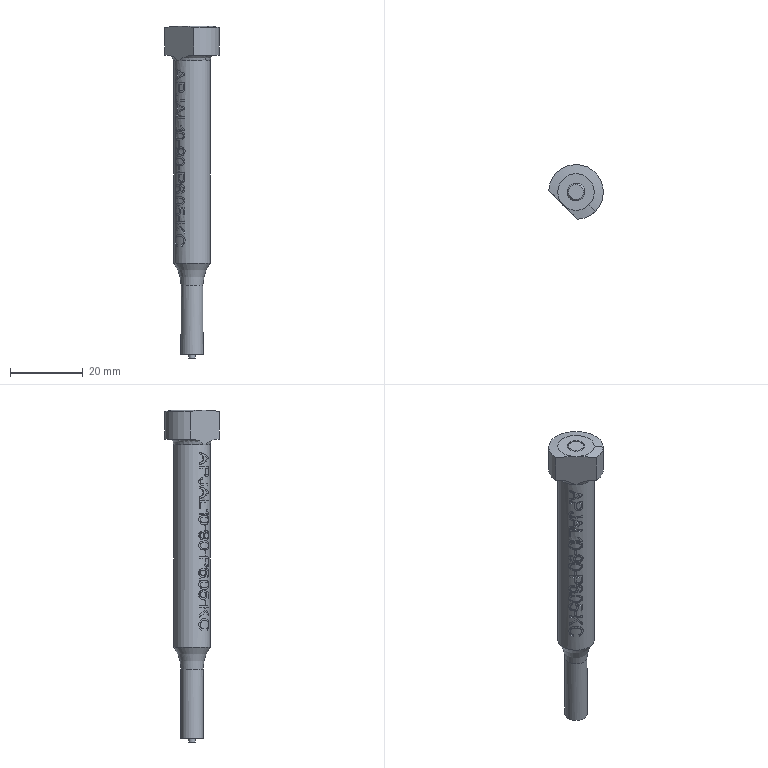Part | NX | features MI_APJAL_0164 2 | 1 solid | 237 faces | box 14.988 x 14.988 x 91 mm | volume 6531 mm3 | plane 140 | cylinder 91 | spline 3 | cone 2 | torus 1 | commonest cylinder face diameters 9.8 x19 10 x10 1.612 x3 1.923 x3 1.929 x3 1.951 x3